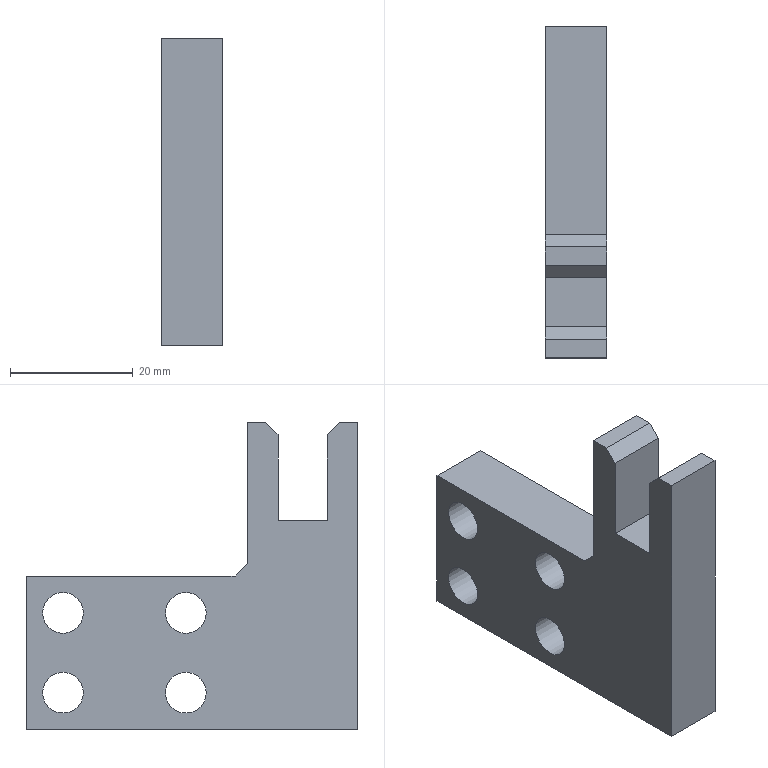Part | NX | features 5003_210_Plate 2 | 1 solid | 19 faces | box 10 x 54.006 x 50 mm | volume 15313 mm3 | plane 15 | cylinder 4 | commonest cylinder face diameters 6.647 x4
STEP:
#1=CARTESIAN_POINT('',(-196.775,-603.606,-138.5));
#2=VERTEX_POINT('',#1);
#3=CARTESIAN_POINT('',(-196.775,-603.606,-115.5));
#4=VERTEX_POINT('',#3);
#5=CARTESIAN_POINT('',(-196.775,-603.606,-140.5));
#6=DIRECTION('',(0.,0.,1.));
#7=VECTOR('',#6,1000.);
#8=LINE('',#5,#7);
#9=EDGE_CURVE('',#2,#4,#8,.T.);
#10=ORIENTED_EDGE('',*,*,#9,.F.);
#11=CARTESIAN_POINT('',(-206.775,-603.606,-138.5));
#12=VERTEX_POINT('',#11);
#13=CARTESIAN_POINT('',(-206.775,-603.606,-138.5));
#14=DIRECTION('',(-1.,0.,0.));
#15=VECTOR('',#14,1000.);
#16=LINE('',#13,#15);
#17=EDGE_CURVE('',#2,#12,#16,.T.);
#18=ORIENTED_EDGE('',*,*,#17,.T.);
#19=CARTESIAN_POINT('',(-206.775,-603.606,-115.5));
#20=VERTEX_POINT('',#19);
#21=CARTESIAN_POINT('',(-206.775,-603.606,-140.5));
#22=DIRECTION('',(0.,0.,1.));
#23=VECTOR('',#22,1000.);
#24=LINE('',#21,#23);
#25=EDGE_CURVE('',#12,#20,#24,.T.);
#26=ORIENTED_EDGE('',*,*,#25,.T.);
#27=CARTESIAN_POINT('',(-196.775,-603.606,-115.5));
#28=DIRECTION('',(-1.,0.,0.));
#29=VECTOR('',#28,1000.);
#30=LINE('',#27,#29);
#31=EDGE_CURVE('',#4,#20,#30,.T.);
#32=ORIENTED_EDGE('',*,*,#31,.F.);
#33=EDGE_LOOP('',(#10,#18,#26,#32));
#34=FACE_BOUND('',#33,.T.);
#35=CARTESIAN_POINT('',(-196.775,-603.606,-140.5));
#36=DIRECTION('',(0.,-1.,0.));
#37=DIRECTION('',(1.,0.,0.));
#38=AXIS2_PLACEMENT_3D('',#35,#36,#37);
#39=PLANE('',#38);
#40=ADVANCED_FACE('',(#34),#39,.F.);
#41=CARTESIAN_POINT('',(-206.775,-606.606,-115.5));
#42=VERTEX_POINT('',#41);
#43=CARTESIAN_POINT('',(-206.775,-603.606,-115.5));
#44=DIRECTION('',(0.,-1.,0.));
#45=VECTOR('',#44,1000.);
#46=LINE('',#43,#45);
#47=EDGE_CURVE('',#20,#42,#46,.T.);
#48=ORIENTED_EDGE('',*,*,#47,.T.);
#49=CARTESIAN_POINT('',(-196.775,-606.606,-115.5));
#50=VERTEX_POINT('',#49);
#51=CARTESIAN_POINT('',(-196.775,-606.606,-115.5));
#52=DIRECTION('',(1.,0.,0.));
#53=VECTOR('',#52,1000.);
#54=LINE('',#51,#53);
#55=EDGE_CURVE('',#42,#50,#54,.T.);
#56=ORIENTED_EDGE('',*,*,#55,.T.);
#57=CARTESIAN_POINT('',(-196.775,-603.606,-115.5));
#58=DIRECTION('',(0.,-1.,0.));
#59=VECTOR('',#58,1000.);
#60=LINE('',#57,#59);
#61=EDGE_CURVE('',#4,#50,#60,.T.);
#62=ORIENTED_EDGE('',*,*,#61,.F.);
#63=ORIENTED_EDGE('',*,*,#31,.T.);
#64=EDGE_LOOP('',(#48,#56,#62,#63));
#65=FACE_BOUND('',#64,.T.);
#66=CARTESIAN_POINT('',(-196.775,-603.606,-115.5));
#67=DIRECTION('',(0.,0.,-1.));
#68=DIRECTION('',(0.,1.,0.));
#69=AXIS2_PLACEMENT_3D('',#66,#67,#68);
#70=PLANE('',#69);
#71=ADVANCED_FACE('',(#65),#70,.F.);
#72=CARTESIAN_POINT('',(-196.775,-608.606,-117.5));
#73=VERTEX_POINT('',#72);
#74=CARTESIAN_POINT('',(-196.775,-608.606,-131.5));
#75=VERTEX_POINT('',#74);
#76=CARTESIAN_POINT('',(-196.775,-608.606,-115.5));
#77=DIRECTION('',(0.,0.,-1.));
#78=VECTOR('',#77,1000.);
#79=LINE('',#76,#78);
#80=EDGE_CURVE('',#73,#75,#79,.T.);
#81=ORIENTED_EDGE('',*,*,#80,.F.);
#82=CARTESIAN_POINT('',(-206.775,-608.606,-117.5));
#83=VERTEX_POINT('',#82);
#84=CARTESIAN_POINT('',(-196.775,-608.606,-117.5));
#85=DIRECTION('',(-1.,0.,0.));
#86=VECTOR('',#85,1000.);
#87=LINE('',#84,#86);
#88=EDGE_CURVE('',#73,#83,#87,.T.);
#89=ORIENTED_EDGE('',*,*,#88,.T.);
#90=CARTESIAN_POINT('',(-206.775,-608.606,-131.5));
#91=VERTEX_POINT('',#90);
#92=CARTESIAN_POINT('',(-206.775,-608.606,-115.5));
#93=DIRECTION('',(0.,0.,-1.));
#94=VECTOR('',#93,1000.);
#95=LINE('',#92,#94);
#96=EDGE_CURVE('',#83,#91,#95,.T.);
#97=ORIENTED_EDGE('',*,*,#96,.T.);
#98=CARTESIAN_POINT('',(-196.775,-608.606,-131.5));
#99=DIRECTION('',(-1.,0.,0.));
#100=VECTOR('',#99,1000.);
#101=LINE('',#98,#100);
#102=EDGE_CURVE('',#75,#91,#101,.T.);
#103=ORIENTED_EDGE('',*,*,#102,.F.);
#104=EDGE_LOOP('',(#81,#89,#97,#103));
#105=FACE_BOUND('',#104,.T.);
#106=CARTESIAN_POINT('',(-196.775,-608.606,-115.5));
#107=DIRECTION('',(0.,1.,0.));
#108=DIRECTION('',(-1.,0.,0.));
#109=AXIS2_PLACEMENT_3D('',#106,#107,#108);
#110=PLANE('',#109);
#111=ADVANCED_FACE('',(#105),#110,.F.);
#112=CARTESIAN_POINT('',(-206.775,-616.606,-131.5));
#113=VERTEX_POINT('',#112);
#114=CARTESIAN_POINT('',(-206.775,-608.606,-131.5));
#115=DIRECTION('',(0.,-1.,0.));
#116=VECTOR('',#115,1000.);
#117=LINE('',#114,#116);
#118=EDGE_CURVE('',#91,#113,#117,.T.);
#119=ORIENTED_EDGE('',*,*,#118,.T.);
#120=CARTESIAN_POINT('',(-196.775,-616.606,-131.5));
#121=VERTEX_POINT('',#120);
#122=CARTESIAN_POINT('',(-196.775,-616.606,-131.5));
#123=DIRECTION('',(-1.,0.,0.));
#124=VECTOR('',#123,1000.);
#125=LINE('',#122,#124);
#126=EDGE_CURVE('',#121,#113,#125,.T.);
#127=ORIENTED_EDGE('',*,*,#126,.F.);
#128=CARTESIAN_POINT('',(-196.775,-608.606,-131.5));
#129=DIRECTION('',(0.,-1.,0.));
#130=VECTOR('',#129,1000.);
#131=LINE('',#128,#130);
#132=EDGE_CURVE('',#75,#121,#131,.T.);
#133=ORIENTED_EDGE('',*,*,#132,.F.);
#134=ORIENTED_EDGE('',*,*,#102,.T.);
#135=EDGE_LOOP('',(#119,#127,#133,#134));
#136=FACE_BOUND('',#135,.T.);
#137=CARTESIAN_POINT('',(-196.775,-608.606,-131.5));
#138=DIRECTION('',(0.,0.,-1.));
#139=DIRECTION('',(0.,1.,0.));
#140=AXIS2_PLACEMENT_3D('',#137,#138,#139);
#141=PLANE('',#140);
#142=ADVANCED_FACE('',(#136),#141,.F.);
#143=CARTESIAN_POINT('',(-206.775,-616.606,-117.5));
#144=VERTEX_POINT('',#143);
#145=CARTESIAN_POINT('',(-206.775,-616.606,-131.5));
#146=DIRECTION('',(0.,0.,1.));
#147=VECTOR('',#146,1000.);
#148=LINE('',#145,#147);
#149=EDGE_CURVE('',#113,#144,#148,.T.);
#150=ORIENTED_EDGE('',*,*,#149,.T.);
#151=CARTESIAN_POINT('',(-196.775,-616.606,-117.5));
#152=VERTEX_POINT('',#151);
#153=CARTESIAN_POINT('',(-196.775,-616.606,-117.5));
#154=DIRECTION('',(1.,0.,0.));
#155=VECTOR('',#154,1000.);
#156=LINE('',#153,#155);
#157=EDGE_CURVE('',#144,#152,#156,.T.);
#158=ORIENTED_EDGE('',*,*,#157,.T.);
#159=CARTESIAN_POINT('',(-196.775,-616.606,-131.5));
#160=DIRECTION('',(0.,0.,1.));
#161=VECTOR('',#160,1000.);
#162=LINE('',#159,#161);
#163=EDGE_CURVE('',#121,#152,#162,.T.);
#164=ORIENTED_EDGE('',*,*,#163,.F.);
#165=ORIENTED_EDGE('',*,*,#126,.T.);
#166=EDGE_LOOP('',(#150,#158,#164,#165));
#167=FACE_BOUND('',#166,.T.);
#168=CARTESIAN_POINT('',(-196.775,-616.606,-131.5));
#169=DIRECTION('',(0.,-1.,0.));
#170=DIRECTION('',(0.,0.,-1.));
#171=AXIS2_PLACEMENT_3D('',#168,#169,#170);
#172=PLANE('',#171);
#173=ADVANCED_FACE('',(#167),#172,.F.);
#174=CARTESIAN_POINT('',(-196.775,-618.606,-115.5));
#175=VERTEX_POINT('',#174);
#176=CARTESIAN_POINT('',(-196.775,-621.606,-115.5));
#177=VERTEX_POINT('',#176);
#178=CARTESIAN_POINT('',(-196.775,-621.606,-115.5));
#179=DIRECTION('',(0.,-1.,0.));
#180=VECTOR('',#179,1000.);
#181=LINE('',#178,#180);
#182=EDGE_CURVE('',#175,#177,#181,.T.);
#183=ORIENTED_EDGE('',*,*,#182,.F.);
#184=CARTESIAN_POINT('',(-206.775,-618.606,-115.5));
#185=VERTEX_POINT('',#184);
#186=CARTESIAN_POINT('',(-196.775,-618.606,-115.5));
#187=DIRECTION('',(-1.,0.,0.));
#188=VECTOR('',#187,1000.);
#189=LINE('',#186,#188);
#190=EDGE_CURVE('',#175,#185,#189,.T.);
#191=ORIENTED_EDGE('',*,*,#190,.T.);
#192=CARTESIAN_POINT('',(-206.775,-621.606,-115.5));
#193=VERTEX_POINT('',#192);
#194=CARTESIAN_POINT('',(-206.775,-621.606,-115.5));
#195=DIRECTION('',(0.,-1.,0.));
#196=VECTOR('',#195,1000.);
#197=LINE('',#194,#196);
#198=EDGE_CURVE('',#185,#193,#197,.T.);
#199=ORIENTED_EDGE('',*,*,#198,.T.);
#200=CARTESIAN_POINT('',(-196.775,-621.606,-115.5));
#201=DIRECTION('',(-1.,0.,0.));
#202=VECTOR('',#201,1000.);
#203=LINE('',#200,#202);
#204=EDGE_CURVE('',#177,#193,#203,.T.);
#205=ORIENTED_EDGE('',*,*,#204,.F.);
#206=EDGE_LOOP('',(#183,#191,#199,#205));
#207=FACE_BOUND('',#206,.T.);
#208=CARTESIAN_POINT('',(-196.775,-621.606,-115.5));
#209=DIRECTION('',(0.,0.,-1.));
#210=DIRECTION('',(0.,1.,0.));
#211=AXIS2_PLACEMENT_3D('',#208,#209,#210);
#212=PLANE('',#211);
#213=ADVANCED_FACE('',(#207),#212,.F.);
#214=CARTESIAN_POINT('',(-206.775,-621.606,-165.5));
#215=VERTEX_POINT('',#214);
#216=CARTESIAN_POINT('',(-206.775,-621.606,-115.5));
#217=DIRECTION('',(0.,0.,-1.));
#218=VECTOR('',#217,1000.);
#219=LINE('',#216,#218);
#220=EDGE_CURVE('',#193,#215,#219,.T.);
#221=ORIENTED_EDGE('',*,*,#220,.T.);
#222=CARTESIAN_POINT('',(-196.775,-621.606,-165.5));
#223=VERTEX_POINT('',#222);
#224=CARTESIAN_POINT('',(-196.775,-621.606,-165.5));
#225=DIRECTION('',(-1.,0.,0.));
#226=VECTOR('',#225,1000.);
#227=LINE('',#224,#226);
#228=EDGE_CURVE('',#223,#215,#227,.T.);
#229=ORIENTED_EDGE('',*,*,#228,.F.);
#230=CARTESIAN_POINT('',(-196.775,-621.606,-115.5));
#231=DIRECTION('',(0.,0.,-1.));
#232=VECTOR('',#231,1000.);
#233=LINE('',#230,#232);
#234=EDGE_CURVE('',#177,#223,#233,.T.);
#235=ORIENTED_EDGE('',*,*,#234,.F.);
#236=ORIENTED_EDGE('',*,*,#204,.T.);
#237=EDGE_LOOP('',(#221,#229,#235,#236));
#238=FACE_BOUND('',#237,.T.);
#239=CARTESIAN_POINT('',(-196.775,-621.606,-115.5));
#240=DIRECTION('',(0.,1.,0.));
#241=DIRECTION('',(-1.,0.,0.));
#242=AXIS2_PLACEMENT_3D('',#239,#240,#241);
#243=PLANE('',#242);
#244=ADVANCED_FACE('',(#238),#243,.F.);
#245=CARTESIAN_POINT('',(-206.775,-567.6,-165.5));
#246=VERTEX_POINT('',#245);
#247=CARTESIAN_POINT('',(-206.775,-621.606,-165.5));
#248=DIRECTION('',(0.,1.,0.));
#249=VECTOR('',#248,1000.);
#250=LINE('',#247,#249);
#251=EDGE_CURVE('',#215,#246,#250,.T.);
#252=ORIENTED_EDGE('',*,*,#251,.T.);
#253=CARTESIAN_POINT('',(-196.775,-567.6,-165.5));
#254=VERTEX_POINT('',#253);
#255=CARTESIAN_POINT('',(-196.775,-567.6,-165.5));
#256=DIRECTION('',(-1.,0.,0.));
#257=VECTOR('',#256,1000.);
#258=LINE('',#255,#257);
#259=EDGE_CURVE('',#254,#246,#258,.T.);
#260=ORIENTED_EDGE('',*,*,#259,.F.);
#261=CARTESIAN_POINT('',(-196.775,-621.606,-165.5));
#262=DIRECTION('',(0.,1.,0.));
#263=VECTOR('',#262,1000.);
#264=LINE('',#261,#263);
#265=EDGE_CURVE('',#223,#254,#264,.T.);
#266=ORIENTED_EDGE('',*,*,#265,.F.);
#267=ORIENTED_EDGE('',*,*,#228,.T.);
#268=EDGE_LOOP('',(#252,#260,#266,#267));
#269=FACE_BOUND('',#268,.T.);
#270=CARTESIAN_POINT('',(-196.775,-621.606,-165.5));
#271=DIRECTION('',(0.,0.,1.));
#272=DIRECTION('',(0.,-1.,0.));
#273=AXIS2_PLACEMENT_3D('',#270,#271,#272);
#274=PLANE('',#273);
#275=ADVANCED_FACE('',(#269),#274,.F.);
#276=CARTESIAN_POINT('',(-206.775,-567.6,-140.5));
#277=VERTEX_POINT('',#276);
#278=CARTESIAN_POINT('',(-206.775,-567.6,-165.5));
#279=DIRECTION('',(0.,0.,1.));
#280=VECTOR('',#279,1000.);
#281=LINE('',#278,#280);
#282=EDGE_CURVE('',#246,#277,#281,.T.);
#283=ORIENTED_EDGE('',*,*,#282,.T.);
#284=CARTESIAN_POINT('',(-196.775,-567.6,-140.5));
#285=VERTEX_POINT('',#284);
#286=CARTESIAN_POINT('',(-196.775,-567.6,-140.5));
#287=DIRECTION('',(-1.,0.,0.));
#288=VECTOR('',#287,1000.);
#289=LINE('',#286,#288);
#290=EDGE_CURVE('',#285,#277,#289,.T.);
#291=ORIENTED_EDGE('',*,*,#290,.F.);
#292=CARTESIAN_POINT('',(-196.775,-567.6,-165.5));
#293=DIRECTION('',(0.,0.,1.));
#294=VECTOR('',#293,1000.);
#295=LINE('',#292,#294);
#296=EDGE_CURVE('',#254,#285,#295,.T.);
#297=ORIENTED_EDGE('',*,*,#296,.F.);
#298=ORIENTED_EDGE('',*,*,#259,.T.);
#299=EDGE_LOOP('',(#283,#291,#297,#298));
#300=FACE_BOUND('',#299,.T.);
#301=CARTESIAN_POINT('',(-196.775,-567.6,-165.5));
#302=DIRECTION('',(0.,-1.,0.));
#303=DIRECTION('',(1.,0.,0.));
#304=AXIS2_PLACEMENT_3D('',#301,#302,#303);
#305=PLANE('',#304);
#306=ADVANCED_FACE('',(#300),#305,.F.);
#307=CARTESIAN_POINT('',(-206.775,-601.606,-140.5));
#308=VERTEX_POINT('',#307);
#309=CARTESIAN_POINT('',(-206.775,-567.6,-140.5));
#310=DIRECTION('',(0.,-1.,0.));
#311=VECTOR('',#310,1000.);
#312=LINE('',#309,#311);
#313=EDGE_CURVE('',#277,#308,#312,.T.);
#314=ORIENTED_EDGE('',*,*,#313,.T.);
#315=CARTESIAN_POINT('',(-196.775,-601.606,-140.5));
#316=VERTEX_POINT('',#315);
#317=CARTESIAN_POINT('',(-196.775,-601.606,-140.5));
#318=DIRECTION('',(1.,0.,0.));
#319=VECTOR('',#318,1000.);
#320=LINE('',#317,#319);
#321=EDGE_CURVE('',#308,#316,#320,.T.);
#322=ORIENTED_EDGE('',*,*,#321,.T.);
#323=CARTESIAN_POINT('',(-196.775,-567.6,-140.5));
#324=DIRECTION('',(0.,-1.,0.));
#325=VECTOR('',#324,1000.);
#326=LINE('',#323,#325);
#327=EDGE_CURVE('',#285,#316,#326,.T.);
#328=ORIENTED_EDGE('',*,*,#327,.F.);
#329=ORIENTED_EDGE('',*,*,#290,.T.);
#330=EDGE_LOOP('',(#314,#322,#328,#329));
#331=FACE_BOUND('',#330,.T.);
#332=CARTESIAN_POINT('',(-196.775,-567.6,-140.5));
#333=DIRECTION('',(0.,0.,-1.));
#334=DIRECTION('',(0.,1.,0.));
#335=AXIS2_PLACEMENT_3D('',#332,#333,#334);
#336=PLANE('',#335);
#337=ADVANCED_FACE('',(#331),#336,.F.);
#338=CARTESIAN_POINT('',(-196.775,-570.276,-146.5));
#339=VERTEX_POINT('',#338);
#340=CARTESIAN_POINT('',(-196.775,-573.6,-146.5));
#341=DIRECTION('',(1.,0.,0.));
#342=DIRECTION('',(0.,1.,0.));
#343=AXIS2_PLACEMENT_3D('',#340,#341,#342);
#344=CIRCLE('',#343,3.324);
#345=EDGE_CURVE('',#339,#339,#344,.T.);
#346=ORIENTED_EDGE('',*,*,#345,.F.);
#347=EDGE_LOOP('',(#346));
#348=FACE_BOUND('',#347,.T.);
#349=CARTESIAN_POINT('',(-196.775,-570.276,-159.5));
#350=VERTEX_POINT('',#349);
#351=CARTESIAN_POINT('',(-196.775,-573.6,-159.5));
#352=DIRECTION('',(1.,0.,0.));
#353=DIRECTION('',(0.,1.,0.));
#354=AXIS2_PLACEMENT_3D('',#351,#352,#353);
#355=CIRCLE('',#354,3.324);
#356=EDGE_CURVE('',#350,#350,#355,.T.);
#357=ORIENTED_EDGE('',*,*,#356,.F.);
#358=EDGE_LOOP('',(#357));
#359=FACE_BOUND('',#358,.T.);
#360=CARTESIAN_POINT('',(-196.775,-590.276,-159.5));
#361=VERTEX_POINT('',#360);
#362=CARTESIAN_POINT('',(-196.775,-593.6,-159.5));
#363=DIRECTION('',(1.,0.,0.));
#364=DIRECTION('',(0.,1.,0.));
#365=AXIS2_PLACEMENT_3D('',#362,#363,#364);
#366=CIRCLE('',#365,3.324);
#367=EDGE_CURVE('',#361,#361,#366,.T.);
#368=ORIENTED_EDGE('',*,*,#367,.F.);
#369=EDGE_LOOP('',(#368));
#370=FACE_BOUND('',#369,.T.);
#371=CARTESIAN_POINT('',(-196.775,-590.276,-146.5));
#372=VERTEX_POINT('',#371);
#373=CARTESIAN_POINT('',(-196.775,-593.6,-146.5));
#374=DIRECTION('',(1.,0.,0.));
#375=DIRECTION('',(0.,1.,0.));
#376=AXIS2_PLACEMENT_3D('',#373,#374,#375);
#377=CIRCLE('',#376,3.324);
#378=EDGE_CURVE('',#372,#372,#377,.T.);
#379=ORIENTED_EDGE('',*,*,#378,.F.);
#380=EDGE_LOOP('',(#379));
#381=FACE_BOUND('',#380,.T.);
#382=ORIENTED_EDGE('',*,*,#61,.T.);
#383=CARTESIAN_POINT('',(-196.775,-639.106,-148.));
#384=DIRECTION('',(0.,0.7071,0.7071));
#385=VECTOR('',#384,1000.);
#386=LINE('',#383,#385);
#387=EDGE_CURVE('',#50,#73,#386,.F.);
#388=ORIENTED_EDGE('',*,*,#387,.T.);
#389=ORIENTED_EDGE('',*,*,#80,.T.);
#390=ORIENTED_EDGE('',*,*,#132,.T.);
#391=ORIENTED_EDGE('',*,*,#163,.T.);
#392=CARTESIAN_POINT('',(-196.775,-595.106,-139.));
#393=DIRECTION('',(0.,0.7071,-0.7071));
#394=VECTOR('',#393,1000.);
#395=LINE('',#392,#394);
#396=EDGE_CURVE('',#152,#175,#395,.F.);
#397=ORIENTED_EDGE('',*,*,#396,.T.);
#398=ORIENTED_EDGE('',*,*,#182,.T.);
#399=ORIENTED_EDGE('',*,*,#234,.T.);
#400=ORIENTED_EDGE('',*,*,#265,.T.);
#401=ORIENTED_EDGE('',*,*,#296,.T.);
#402=ORIENTED_EDGE('',*,*,#327,.T.);
#403=CARTESIAN_POINT('',(-196.775,-603.606,-138.5));
#404=DIRECTION('',(0.,0.7071,-0.7071));
#405=VECTOR('',#404,1000.);
#406=LINE('',#403,#405);
#407=EDGE_CURVE('',#316,#2,#406,.F.);
#408=ORIENTED_EDGE('',*,*,#407,.T.);
#409=ORIENTED_EDGE('',*,*,#9,.T.);
#410=EDGE_LOOP('',(#382,#388,#389,#390,#391,#397,#398,#399,#400,#401,#402,#408,#409));
#411=FACE_BOUND('',#410,.T.);
#412=CARTESIAN_POINT('',(-196.775,-621.606,-165.5));
#413=DIRECTION('',(1.,0.,0.));
#414=DIRECTION('',(0.,1.,0.));
#415=AXIS2_PLACEMENT_3D('',#412,#413,#414);
#416=PLANE('',#415);
#417=ADVANCED_FACE('',(#348,#359,#370,#381,#411),#416,.T.);
#418=CARTESIAN_POINT('',(-206.775,-570.276,-146.5));
#419=VERTEX_POINT('',#418);
#420=CARTESIAN_POINT('',(-206.775,-573.6,-146.5));
#421=DIRECTION('',(1.,0.,0.));
#422=DIRECTION('',(0.,1.,0.));
#423=AXIS2_PLACEMENT_3D('',#420,#421,#422);
#424=CIRCLE('',#423,3.324);
#425=EDGE_CURVE('',#419,#419,#424,.T.);
#426=ORIENTED_EDGE('',*,*,#425,.T.);
#427=EDGE_LOOP('',(#426));
#428=FACE_BOUND('',#427,.T.);
#429=CARTESIAN_POINT('',(-206.775,-570.276,-159.5));
#430=VERTEX_POINT('',#429);
#431=CARTESIAN_POINT('',(-206.775,-573.6,-159.5));
#432=DIRECTION('',(1.,0.,0.));
#433=DIRECTION('',(0.,1.,0.));
#434=AXIS2_PLACEMENT_3D('',#431,#432,#433);
#435=CIRCLE('',#434,3.324);
#436=EDGE_CURVE('',#430,#430,#435,.T.);
#437=ORIENTED_EDGE('',*,*,#436,.T.);
#438=EDGE_LOOP('',(#437));
#439=FACE_BOUND('',#438,.T.);
#440=CARTESIAN_POINT('',(-206.775,-590.276,-159.5));
#441=VERTEX_POINT('',#440);
#442=CARTESIAN_POINT('',(-206.775,-593.6,-159.5));
#443=DIRECTION('',(1.,0.,0.));
#444=DIRECTION('',(0.,1.,0.));
#445=AXIS2_PLACEMENT_3D('',#442,#443,#444);
#446=CIRCLE('',#445,3.324);
#447=EDGE_CURVE('',#441,#441,#446,.T.);
#448=ORIENTED_EDGE('',*,*,#447,.T.);
#449=EDGE_LOOP('',(#448));
#450=FACE_BOUND('',#449,.T.);
#451=CARTESIAN_POINT('',(-206.775,-590.276,-146.5));
#452=VERTEX_POINT('',#451);
#453=CARTESIAN_POINT('',(-206.775,-593.6,-146.5));
#454=DIRECTION('',(1.,0.,0.));
#455=DIRECTION('',(0.,1.,0.));
#456=AXIS2_PLACEMENT_3D('',#453,#454,#455);
#457=CIRCLE('',#456,3.324);
#458=EDGE_CURVE('',#452,#452,#457,.T.);
#459=ORIENTED_EDGE('',*,*,#458,.T.);
#460=EDGE_LOOP('',(#459));
#461=FACE_BOUND('',#460,.T.);
#462=ORIENTED_EDGE('',*,*,#96,.F.);
#463=CARTESIAN_POINT('',(-206.775,-608.606,-117.5));
#464=DIRECTION('',(0.,-0.7071,-0.7071));
#465=VECTOR('',#464,1000.);
#466=LINE('',#463,#465);
#467=EDGE_CURVE('',#83,#42,#466,.F.);
#468=ORIENTED_EDGE('',*,*,#467,.T.);
#469=ORIENTED_EDGE('',*,*,#47,.F.);
#470=ORIENTED_EDGE('',*,*,#25,.F.);
#471=CARTESIAN_POINT('',(-206.775,-599.106,-143.));
#472=DIRECTION('',(0.,-0.7071,0.7071));
#473=VECTOR('',#472,1000.);
#474=LINE('',#471,#473);
#475=EDGE_CURVE('',#12,#308,#474,.F.);
#476=ORIENTED_EDGE('',*,*,#475,.T.);
#477=ORIENTED_EDGE('',*,*,#313,.F.);
#478=ORIENTED_EDGE('',*,*,#282,.F.);
#479=ORIENTED_EDGE('',*,*,#251,.F.);
#480=ORIENTED_EDGE('',*,*,#220,.F.);
#481=ORIENTED_EDGE('',*,*,#198,.F.);
#482=CARTESIAN_POINT('',(-206.775,-618.606,-115.5));
#483=DIRECTION('',(0.,-0.7071,0.7071));
#484=VECTOR('',#483,1000.);
#485=LINE('',#482,#484);
#486=EDGE_CURVE('',#185,#144,#485,.F.);
#487=ORIENTED_EDGE('',*,*,#486,.T.);
#488=ORIENTED_EDGE('',*,*,#149,.F.);
#489=ORIENTED_EDGE('',*,*,#118,.F.);
#490=EDGE_LOOP('',(#462,#468,#469,#470,#476,#477,#478,#479,#480,#481,#487,#488,#489));
#491=FACE_BOUND('',#490,.T.);
#492=CARTESIAN_POINT('',(-206.775,-621.606,-165.5));
#493=DIRECTION('',(1.,0.,0.));
#494=DIRECTION('',(0.,1.,0.));
#495=AXIS2_PLACEMENT_3D('',#492,#493,#494);
#496=PLANE('',#495);
#497=ADVANCED_FACE('',(#428,#439,#450,#461,#491),#496,.F.);
#498=ORIENTED_EDGE('',*,*,#458,.F.);
#499=EDGE_LOOP('',(#498));
#500=FACE_BOUND('',#499,.T.);
#501=ORIENTED_EDGE('',*,*,#378,.T.);
#502=EDGE_LOOP('',(#501));
#503=FACE_BOUND('',#502,.T.);
#504=CARTESIAN_POINT('',(-196.775,-593.6,-146.5));
#505=DIRECTION('',(1.,0.,0.));
#506=DIRECTION('',(0.,1.,0.));
#507=AXIS2_PLACEMENT_3D('',#504,#505,#506);
#508=CYLINDRICAL_SURFACE('',#507,3.324);
#509=ADVANCED_FACE('',(#500,#503),#508,.F.);
#510=ORIENTED_EDGE('',*,*,#447,.F.);
#511=EDGE_LOOP('',(#510));
#512=FACE_BOUND('',#511,.T.);
#513=ORIENTED_EDGE('',*,*,#367,.T.);
#514=EDGE_LOOP('',(#513));
#515=FACE_BOUND('',#514,.T.);
#516=CARTESIAN_POINT('',(-196.775,-593.6,-159.5));
#517=DIRECTION('',(1.,0.,0.));
#518=DIRECTION('',(0.,1.,0.));
#519=AXIS2_PLACEMENT_3D('',#516,#517,#518);
#520=CYLINDRICAL_SURFACE('',#519,3.324);
#521=ADVANCED_FACE('',(#512,#515),#520,.F.);
#522=ORIENTED_EDGE('',*,*,#436,.F.);
#523=EDGE_LOOP('',(#522));
#524=FACE_BOUND('',#523,.T.);
#525=ORIENTED_EDGE('',*,*,#356,.T.);
#526=EDGE_LOOP('',(#525));
#527=FACE_BOUND('',#526,.T.);
#528=CARTESIAN_POINT('',(-196.775,-573.6,-159.5));
#529=DIRECTION('',(1.,0.,0.));
#530=DIRECTION('',(0.,1.,0.));
#531=AXIS2_PLACEMENT_3D('',#528,#529,#530);
#532=CYLINDRICAL_SURFACE('',#531,3.324);
#533=ADVANCED_FACE('',(#524,#527),#532,.F.);
#534=ORIENTED_EDGE('',*,*,#425,.F.);
#535=EDGE_LOOP('',(#534));
#536=FACE_BOUND('',#535,.T.);
#537=ORIENTED_EDGE('',*,*,#345,.T.);
#538=EDGE_LOOP('',(#537));
#539=FACE_BOUND('',#538,.T.);
#540=CARTESIAN_POINT('',(-196.775,-573.6,-146.5));
#541=DIRECTION('',(1.,0.,0.));
#542=DIRECTION('',(0.,1.,0.));
#543=AXIS2_PLACEMENT_3D('',#540,#541,#542);
#544=CYLINDRICAL_SURFACE('',#543,3.324);
#545=ADVANCED_FACE('',(#536,#539),#544,.F.);
#546=ORIENTED_EDGE('',*,*,#407,.F.);
#547=ORIENTED_EDGE('',*,*,#321,.F.);
#548=ORIENTED_EDGE('',*,*,#475,.F.);
#549=ORIENTED_EDGE('',*,*,#17,.F.);
#550=EDGE_LOOP('',(#546,#547,#548,#549));
#551=FACE_BOUND('',#550,.T.);
#552=CARTESIAN_POINT('',(-196.775,-603.606,-138.5));
#553=DIRECTION('',(0.,0.7071,0.7071));
#554=DIRECTION('',(1.,0.,0.));
#555=AXIS2_PLACEMENT_3D('',#552,#553,#554);
#556=PLANE('',#555);
#557=ADVANCED_FACE('',(#551),#556,.T.);
#558=ORIENTED_EDGE('',*,*,#387,.F.);
#559=ORIENTED_EDGE('',*,*,#55,.F.);
#560=ORIENTED_EDGE('',*,*,#467,.F.);
#561=ORIENTED_EDGE('',*,*,#88,.F.);
#562=EDGE_LOOP('',(#558,#559,#560,#561));
#563=FACE_BOUND('',#562,.T.);
#564=CARTESIAN_POINT('',(-196.775,-608.606,-117.5));
#565=DIRECTION('',(0.,0.7071,-0.7071));
#566=DIRECTION('',(-1.,0.,0.));
#567=AXIS2_PLACEMENT_3D('',#564,#565,#566);
#568=PLANE('',#567);
#569=ADVANCED_FACE('',(#563),#568,.F.);
#570=ORIENTED_EDGE('',*,*,#396,.F.);
#571=ORIENTED_EDGE('',*,*,#157,.F.);
#572=ORIENTED_EDGE('',*,*,#486,.F.);
#573=ORIENTED_EDGE('',*,*,#190,.F.);
#574=EDGE_LOOP('',(#570,#571,#572,#573));
#575=FACE_BOUND('',#574,.T.);
#576=CARTESIAN_POINT('',(-196.775,-618.606,-115.5));
#577=DIRECTION('',(0.,-0.7071,-0.7071));
#578=DIRECTION('',(-1.,0.,0.));
#579=AXIS2_PLACEMENT_3D('',#576,#577,#578);
#580=PLANE('',#579);
#581=ADVANCED_FACE('',(#575),#580,.F.);
#582=CLOSED_SHELL('',(#40,#71,#111,#142,#173,#213,#244,#275,#306,#337,#417,#497,#509,#521,#533,#545,#557,#569,#581));
#583=MANIFOLD_SOLID_BREP('',#582);
#584=(LENGTH_UNIT()NAMED_UNIT(*)SI_UNIT(.MILLI.,.METRE.));
#585=UNCERTAINTY_MEASURE_WITH_UNIT(LENGTH_MEASURE(0.00001),#584,'','');
#586=(NAMED_UNIT(*)PLANE_ANGLE_UNIT()SI_UNIT($,.RADIAN.));
#587=(NAMED_UNIT(*)SI_UNIT($,.STERADIAN.)SOLID_ANGLE_UNIT());
#588=(GEOMETRIC_REPRESENTATION_CONTEXT(3)GLOBAL_UNCERTAINTY_ASSIGNED_CONTEXT((#585))GLOBAL_UNIT_ASSIGNED_CONTEXT((#584,#586,#587))REPRESENTATION_CONTEXT('',''));
#589=ADVANCED_BREP_SHAPE_REPRESENTATION('',(#583),#588);